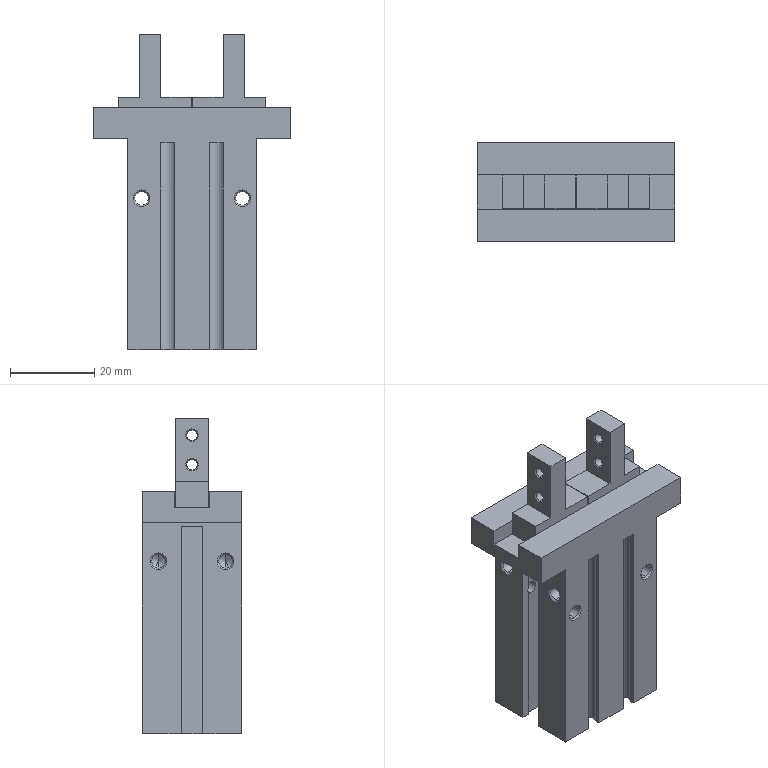Part | STEP file | MHZL2-16S (14.9) | 1 solid | 155 faces | box 47 x 23.6 x 75 mm | volume 38591 mm3 | plane 71 | cone 42 | cylinder 42 | commonest cylinder face diameters 3.24 x16 4.1 x12 2.46 x8 3 x2 4.48 x2 17 x2